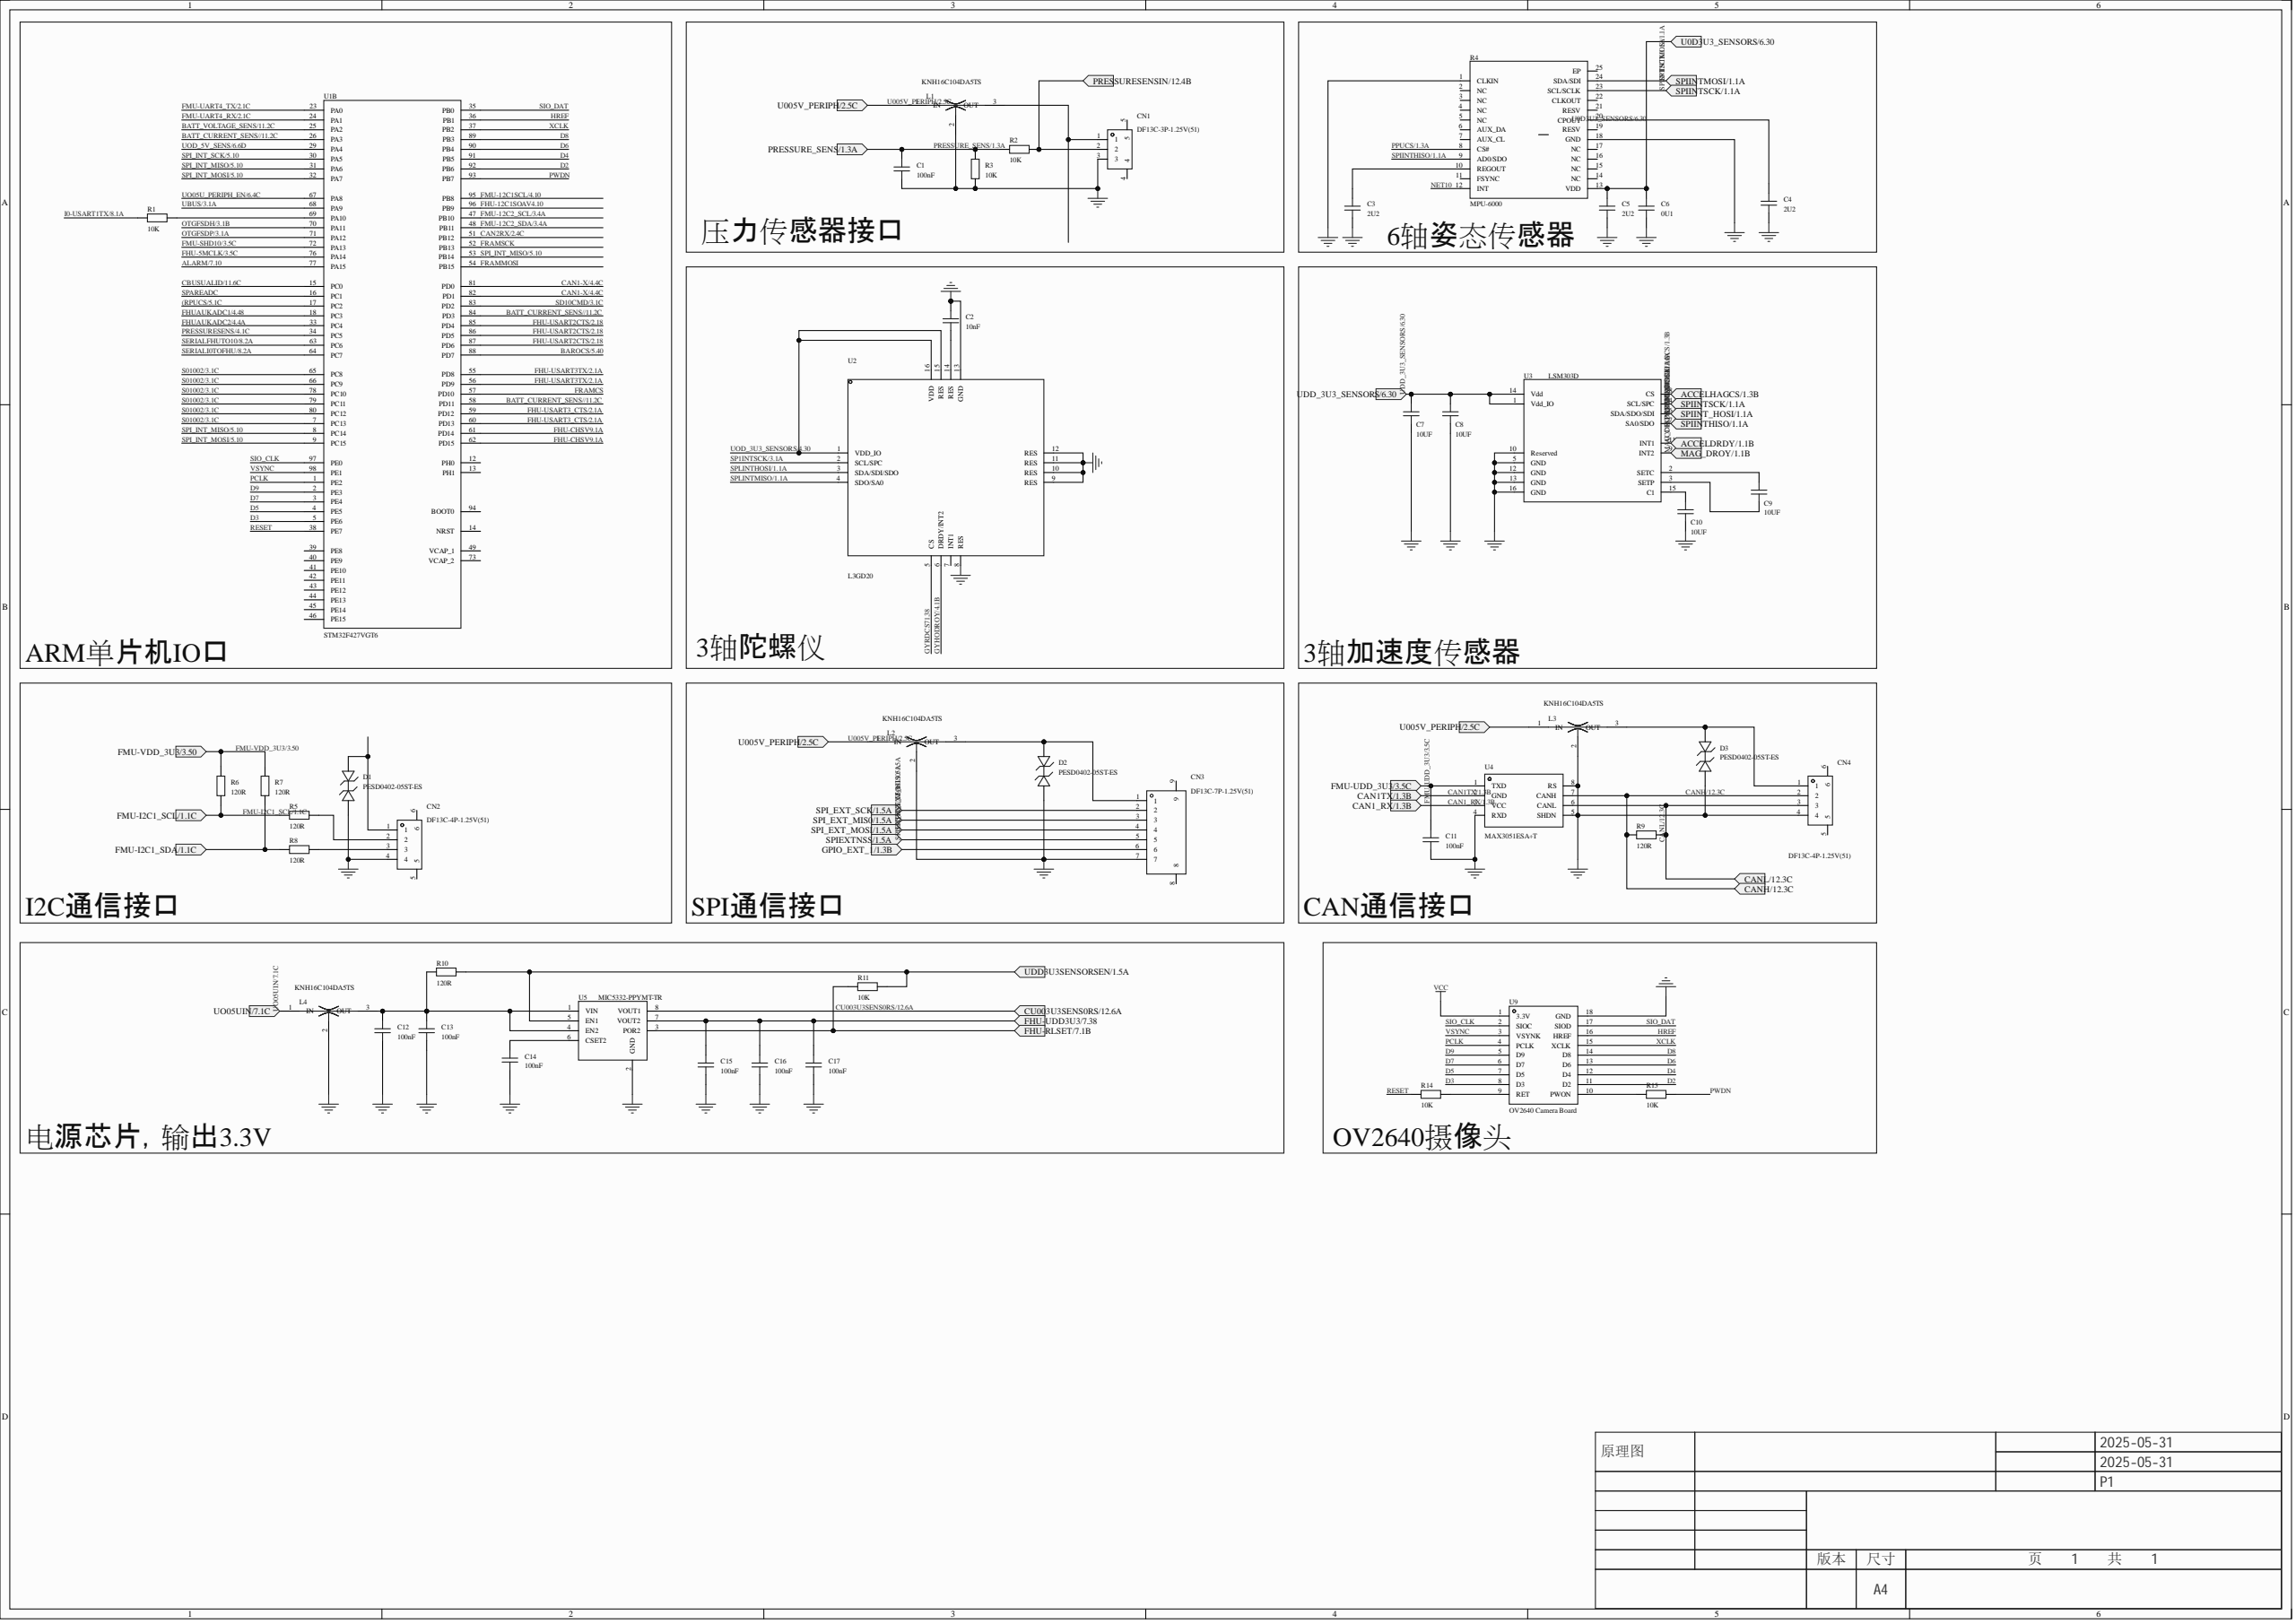Circuit board | Altium Designer | 47 parts | 60 nets
Bill of materials:
Comment,Description,Designator,Footprint,LibRef,Quantity
"100nF","","C1, C11, C12, C13, C14, C15, C16, C17","C0603","CAP_0603","8"
"10nF","","C2","C0603","CAP_0603","1"
"2U2","","C3, C4, C5","C0603","CAP_0603","3"
"0U1","","C6","C0603","CAP_0603","1"
"10UF","","C7, C8, C9, C10","C0603","CAP_0603","4"
"DF13C-3P-1.25V(51)","","CN1","CONN-SMD_3P-P1.25_DF13C-3P-1.25V","DF13C-3P-1.25V(51)","1"
"DF13C-4P-1.25V(51)","","CN2, CN4","CONN-SMD_4P-P1.25_DF13C-4P-1.25V","DF13C-4P-1.25V(51)","2"
"DF13C-7P-1.25V(51)","","CN3","CONN-SMD_7P-P1.25_DF13C-7P-1.25V","DF13C-7P-1.25V(51)","1"
"PESD0402-05ST-ES","","D1, D2, D3","DFN1006-2L-BI","PESD0402-05ST-ES","3"
"KNH16C104DA5TS","","L1, L2, L3, L4","FILTER-SMD_3P-L1.6-W0.8_YFF18PCXXXXXXX","KNH16C104DA5TS_C7435624","4"
"10K","","R1, R2, R3, R11, R14, R15","R0603","Res_0603","6"
"MPU-6000","","R4","QFN-24_L4.0-W4.0-P0.50-BL-EP2.7","MPU-6000","1"
"120R","","R5, R6, R7, R8, R9, R10","R0603","Res_0603","6"
"STM32F427VGT6","","U1","LQFP-100_L14.0-W14.0-P0.50-LS16.0-BL","STM32F427VGT6","1"
"L3GD20","","U2","LGA-16_L4.0-W4.0-P0.65-BL","L3GD20","1"
"LSM303D","","U3","LGA-16_L3.0-W3.0-P0.50-TL","LSM303D","1"
"MAX3051ESA+T","","U4","SOIC-8_L4.9-W3.9-P1.27-LS6.0-BL","MAX3051ESA+T","1"
"MIC5332-PPYMT-TR","","U5","MLF-8_L2.0-W2.0-P0.50-BL-EP","MIC5332-PPYMT-TR","1"
"OV2640 Camera Board","","U9","SENSORM-TH_L35.7-W3.9-OV2640","OV2640 Camera Board","1"
Netlist (Protel format):
[
C1
C0603
100nF



]
[
C2
C0603
10nF



]
[
C3
C0603
2U2



]
[
C4
C0603
2U2



]
[
C5
C0603
2U2



]
[
C6
C0603
0U1



]
[
C7
C0603
10UF



]
[
C8
C0603
10UF



]
[
C9
C0603
10UF



]
[
C10
C0603
10UF



]
[
C11
C0603
100nF



]
[
C12
C0603
100nF



]
[
C13
C0603
100nF



]
[
C14
C0603
100nF



]
[
C15
C0603
100nF



]
[
C16
C0603
100nF



]
[
C17
C0603
100nF



]
[
CN1
CONN-SMD_3P-P1.25_DF13C-3P-1.25V
DF13C-3P-1.25V(51)



]
[
CN2
CONN-SMD_4P-P1.25_DF13C-4P-1.25V
DF13C-4P-1.25V(51)



]
[
CN3
CONN-SMD_7P-P1.25_DF13C-7P-1.25V
DF13C-7P-1.25V(51)



]
[
CN4
CONN-SMD_4P-P1.25_DF13C-4P-1.25V
DF13C-4P-1.25V(51)



]
[
D1
DFN1006-2L-BI
PESD0402-05ST-ES



]
[
D2
DFN1006-2L-BI
PESD0402-05ST-ES



]
[
D3
DFN1006-2L-BI
PESD0402-05ST-ES



]
[
L1
FILTER-SMD_3P-L1.6-W0.8_YFF18PCXXXXXXX
KNH16C104DA5TS



]
[
L2
FILTER-SMD_3P-L1.6-W0.8_YFF18PCXXXXXXX
KNH16C104DA5TS



]
[
L3
FILTER-SMD_3P-L1.6-W0.8_YFF18PCXXXXXXX
KNH16C104DA5TS



]
[
L4
FILTER-SMD_3P-L1.6-W0.8_YFF18PCXXXXXXX
KNH16C104DA5TS



]
[
R1
R0603
10K



]
[
R2
R0603
10K



]
[
R3
R0603
10K



]
[
R4
QFN-24_L4.0-W4.0-P0.50-BL-EP2.7
MPU-6000



]
[
R5
R0603
120R



]
[
R6
R0603
120R



]
[
R7
R0603
120R



]
[
R8
R0603
120R



]
[
R9
R0603
120R



]
[
R10
R0603
120R



]
[
R11
R0603
10K



]
[
R14
R0603
10K



]
[
R15
R0603
10K



]
[
U1
LQFP-100_L14.0-W14.0-P0.50-LS16.0-BL
STM32F427VGT6



]
[
U2
LGA-16_L4.0-W4.0-P0.65-BL
L3GD20



]
[
U3
LGA-16_L3.0-W3.0-P0.50-TL
LSM303D



]
[
U4
SOIC-8_L4.9-W3.9-P1.27-LS6.0-BL
MAX3051ESA+T



]
[
U5
MLF-8_L2.0-W2.0-P0.50-BL-EP
MIC5332-PPYMT-TR



]
[
U9
SENSORM-TH_L35.7-W3.9-OV2640
OV2640 Camera Board



]
(
XCLK
U1-37
U9-15
)
(
VSYNC
U1-98
U9-3
)
(
UOD_3U3_SENSORS/4.30
U2-1
U2-15
U2-16
)
(
UDD_3U3_SENSORS/6.30
C7-2
C8-2
U3-1
U3-14
)
(
U005V_PERIPH/2.5C
L1-1
L2-1
L3-1
)
(
U0D3U3_SENSORS/6.30
C5-2
C6-2
R4-13
)
(
SPIINTSCK/1.1A
R4-23
U3-4
)
(
SPIINTHISO/1.1A
R4-9
U3-7
)
(
SPI_INT_MOSI/5.10
U1-9
U1-32
)
(
SPI_INT_MISO/5.10
U1-8
U1-31
U1-53
)
(
SIO_DAT
U1-35
U9-17
)
(
SIO_CLK
U1-97
U9-2
)
(
S01002/3.1C
U1-7
U1-65
U1-66
U1-78
U1-79
U1-80
)
(
RESET
R14-1
U1-38
)
(
PWDN
R15-2
U1-93
)
(
PRESSURE_SENS/1.3A
C1-2
R2-1
R3-2
)
(
PCLK
U1-1
U9-4
)
(
NetR15_1
R15-1
U9-10
)
(
NetR14_2
R14-2
U9-9
)
(
NetR11_1
R11-1
U5-3
)
(
NetR10_2
R10-2
R11-2
U5-5
)
(
NetR7_1
R7-1
R8-1
)
(
NetR1_2
R1-2
U1-69
)
(
NetCN4_1
CN4-1
D3-2
L3-3
)
(
NetCN3_1
CN3-1
D2-2
L2-3
)
(
NetCN2_3
CN2-3
R8-2
)
(
NetCN2_2
CN2-2
R5-2
)
(
NetCN2_1
CN2-1
D1-2
)
(
NetCN1_2
CN1-2
R2-2
)
(
NetCN1_1
CN1-1
L1-3
)
(
NetC15_2
C15-2
C16-2
C17-2
U5-7
)
(
NetC14_2
C14-2
U5-6
)
(
NetC12_2
C12-2
C13-2
L4-3
R10-1
U5-1
U5-4
)
(
NetC10_2
C10-2
U3-15
)
(
NetC9_2
C9-2
U3-2
)
(
NetC9_1
C9-1
U3-3
)
(
NetC4_2
C4-2
R4-20
)
(
NetC3_2
C3-2
R4-10
)
(
NetC2_1
C2-1
U2-14
)
(
HREF
U1-36
U9-16
)
(
GND
C1-1
C2-2
C3-1
C4-1
C5-1
C6-1
C7-1
C8-1
C10-1
C11-1
C12-1
C13-1
C14-1
C15-1
C16-1
C17-1
CN1-3
CN2-4
CN3-7
CN4-4
D1-1
D2-1
D3-1
L1-2
L2-2
L3-2
L4-2
R3-1
R4-1
R4-18
U2-8
U2-9
U2-10
U2-11
U2-12
U2-13
U3-5
U3-10
U3-12
U3-13
U3-16
U4-4
U4-5
U4-8
U5-2
U9-18
)
(
FMU-VDD_3U3/3.50
R6-2
R7-2
)
(
FMU-UDD_3U3/3.5C
C11-2
U4-1
)
(
FMU-I2C1_SCL/1.1C
R5-1
R6-1
)
(
FHU-USART3TX/2.1A
U1-55
U1-56
)
(
FHU-USART3_CTS/2.1A
U1-59
U1-60
)
(
FHU-USART2CTS/2.18
U1-85
U1-86
U1-87
)
(
FHU-CHSV9.1A
U1-61
U1-62
)
(
D9
U1-2
U9-5
)
(
D8
U1-89
U9-14
)
(
D7
U1-3
U9-6
)
(
D6
U1-90
U9-13
)
(
D5
U1-4
U9-7
)
(
D4
U1-91
U9-12
)
(
D3
U1-5
U9-8
)
(
D2
U1-92
U9-11
)
(
CANL/12.3C
CN4-3
R9-2
U4-6
)
(
CANH/12.3C
CN4-2
R9-1
U4-7
)
(
CAN1-X/4.4C
U1-81
U1-82
)
(
BATT_CURRENT_SENS//11.2C
U1-26
U1-58
U1-84
)